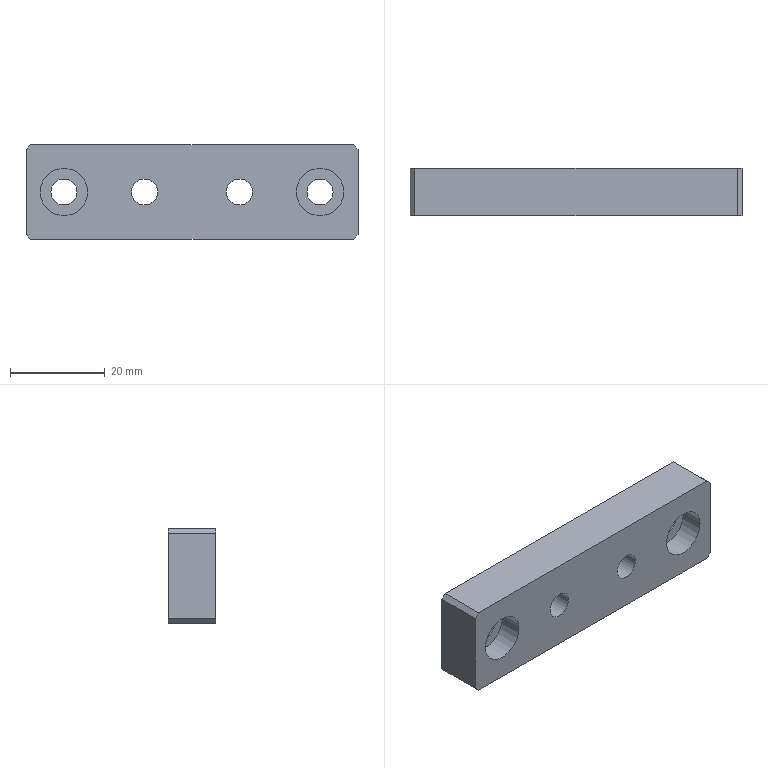Part | SolidWorks | features SplitBody 1 | 1 solid | 30 faces | box 70 x 10 x 20 mm | volume 11934 mm3 | cylinder 16 | plane 14 | commonest cylinder face diameters 5.5 x8 10 x8
STEP:
#1=CARTESIAN_POINT('',(508.292,46.908,-459.936));
#2=VERTEX_POINT('',#1);
#3=CARTESIAN_POINT('',(518.292,46.908,-459.936));
#4=VERTEX_POINT('',#3);
#5=CARTESIAN_POINT('',(513.292,46.908,-459.936));
#6=DIRECTION('',(0.,-1.,0.));
#7=DIRECTION('',(1.,0.,0.));
#8=AXIS2_PLACEMENT_3D('',#5,#6,#7);
#9=CIRCLE('',#8,5.);
#10=EDGE_CURVE('',#2,#4,#9,.T.);
#11=ORIENTED_EDGE('',*,*,#10,.F.);
#12=CARTESIAN_POINT('',(508.292,41.908,-459.936));
#13=VERTEX_POINT('',#12);
#14=CARTESIAN_POINT('',(508.292,41.908,-459.936));
#15=DIRECTION('',(0.,-1.,0.));
#16=VECTOR('',#15,1000.);
#17=LINE('',#14,#16);
#18=EDGE_CURVE('',#2,#13,#17,.T.);
#19=ORIENTED_EDGE('',*,*,#18,.T.);
#20=CARTESIAN_POINT('',(518.292,41.908,-459.936));
#21=VERTEX_POINT('',#20);
#22=CARTESIAN_POINT('',(513.292,41.908,-459.936));
#23=DIRECTION('',(0.,-1.,0.));
#24=DIRECTION('',(1.,0.,0.));
#25=AXIS2_PLACEMENT_3D('',#22,#23,#24);
#26=CIRCLE('',#25,5.);
#27=EDGE_CURVE('',#13,#21,#26,.T.);
#28=ORIENTED_EDGE('',*,*,#27,.T.);
#29=CARTESIAN_POINT('',(518.292,41.908,-459.936));
#30=DIRECTION('',(0.,-1.,0.));
#31=VECTOR('',#30,1000.);
#32=LINE('',#29,#31);
#33=EDGE_CURVE('',#4,#21,#32,.T.);
#34=ORIENTED_EDGE('',*,*,#33,.F.);
#35=EDGE_LOOP('',(#11,#19,#28,#34));
#36=FACE_OUTER_BOUND('',#35,.T.);
#37=CARTESIAN_POINT('',(513.292,41.908,-459.936));
#38=DIRECTION('',(0.,-1.,0.));
#39=DIRECTION('',(1.,0.,0.));
#40=AXIS2_PLACEMENT_3D('',#37,#38,#39);
#41=CYLINDRICAL_SURFACE('',#40,5.);
#42=ADVANCED_FACE('',(#36),#41,.F.);
#43=CARTESIAN_POINT('',(510.542,51.908,-459.936));
#44=VERTEX_POINT('',#43);
#45=CARTESIAN_POINT('',(516.042,51.908,-459.936));
#46=VERTEX_POINT('',#45);
#47=CARTESIAN_POINT('',(513.292,51.908,-459.936));
#48=DIRECTION('',(0.,-1.,0.));
#49=DIRECTION('',(1.,0.,0.));
#50=AXIS2_PLACEMENT_3D('',#47,#48,#49);
#51=CIRCLE('',#50,2.75);
#52=EDGE_CURVE('',#44,#46,#51,.T.);
#53=ORIENTED_EDGE('',*,*,#52,.F.);
#54=CARTESIAN_POINT('',(510.542,46.908,-459.936));
#55=VERTEX_POINT('',#54);
#56=CARTESIAN_POINT('',(510.542,41.908,-459.936));
#57=DIRECTION('',(0.,-1.,0.));
#58=VECTOR('',#57,1000.);
#59=LINE('',#56,#58);
#60=EDGE_CURVE('',#44,#55,#59,.T.);
#61=ORIENTED_EDGE('',*,*,#60,.T.);
#62=CARTESIAN_POINT('',(516.042,46.908,-459.936));
#63=VERTEX_POINT('',#62);
#64=CARTESIAN_POINT('',(513.292,46.908,-459.936));
#65=DIRECTION('',(0.,-1.,0.));
#66=DIRECTION('',(1.,0.,0.));
#67=AXIS2_PLACEMENT_3D('',#64,#65,#66);
#68=CIRCLE('',#67,2.75);
#69=EDGE_CURVE('',#55,#63,#68,.T.);
#70=ORIENTED_EDGE('',*,*,#69,.T.);
#71=CARTESIAN_POINT('',(516.042,41.908,-459.936));
#72=DIRECTION('',(0.,-1.,0.));
#73=VECTOR('',#72,1000.);
#74=LINE('',#71,#73);
#75=EDGE_CURVE('',#46,#63,#74,.T.);
#76=ORIENTED_EDGE('',*,*,#75,.F.);
#77=EDGE_LOOP('',(#53,#61,#70,#76));
#78=FACE_OUTER_BOUND('',#77,.T.);
#79=CARTESIAN_POINT('',(513.292,41.908,-459.936));
#80=DIRECTION('',(0.,-1.,0.));
#81=DIRECTION('',(1.,0.,0.));
#82=AXIS2_PLACEMENT_3D('',#79,#80,#81);
#83=CYLINDRICAL_SURFACE('',#82,2.75);
#84=ADVANCED_FACE('',(#78),#83,.F.);
#85=CARTESIAN_POINT('',(562.292,46.908,-459.936));
#86=VERTEX_POINT('',#85);
#87=CARTESIAN_POINT('',(572.292,46.908,-459.936));
#88=VERTEX_POINT('',#87);
#89=CARTESIAN_POINT('',(567.292,46.908,-459.936));
#90=DIRECTION('',(0.,-1.,0.));
#91=DIRECTION('',(1.,0.,0.));
#92=AXIS2_PLACEMENT_3D('',#89,#90,#91);
#93=CIRCLE('',#92,5.);
#94=EDGE_CURVE('',#86,#88,#93,.T.);
#95=ORIENTED_EDGE('',*,*,#94,.F.);
#96=CARTESIAN_POINT('',(562.292,41.908,-459.936));
#97=VERTEX_POINT('',#96);
#98=CARTESIAN_POINT('',(562.292,41.908,-459.936));
#99=DIRECTION('',(0.,-1.,0.));
#100=VECTOR('',#99,1000.);
#101=LINE('',#98,#100);
#102=EDGE_CURVE('',#86,#97,#101,.T.);
#103=ORIENTED_EDGE('',*,*,#102,.T.);
#104=CARTESIAN_POINT('',(572.292,41.908,-459.936));
#105=VERTEX_POINT('',#104);
#106=CARTESIAN_POINT('',(567.292,41.908,-459.936));
#107=DIRECTION('',(0.,-1.,0.));
#108=DIRECTION('',(1.,0.,0.));
#109=AXIS2_PLACEMENT_3D('',#106,#107,#108);
#110=CIRCLE('',#109,5.);
#111=EDGE_CURVE('',#97,#105,#110,.T.);
#112=ORIENTED_EDGE('',*,*,#111,.T.);
#113=CARTESIAN_POINT('',(572.292,41.908,-459.936));
#114=DIRECTION('',(0.,-1.,0.));
#115=VECTOR('',#114,1000.);
#116=LINE('',#113,#115);
#117=EDGE_CURVE('',#88,#105,#116,.T.);
#118=ORIENTED_EDGE('',*,*,#117,.F.);
#119=EDGE_LOOP('',(#95,#103,#112,#118));
#120=FACE_OUTER_BOUND('',#119,.T.);
#121=CARTESIAN_POINT('',(567.292,41.908,-459.936));
#122=DIRECTION('',(0.,-1.,0.));
#123=DIRECTION('',(1.,0.,0.));
#124=AXIS2_PLACEMENT_3D('',#121,#122,#123);
#125=CYLINDRICAL_SURFACE('',#124,5.);
#126=ADVANCED_FACE('',(#120),#125,.F.);
#127=CARTESIAN_POINT('',(564.542,51.908,-459.936));
#128=VERTEX_POINT('',#127);
#129=CARTESIAN_POINT('',(570.042,51.908,-459.936));
#130=VERTEX_POINT('',#129);
#131=CARTESIAN_POINT('',(567.292,51.908,-459.936));
#132=DIRECTION('',(0.,-1.,0.));
#133=DIRECTION('',(1.,0.,0.));
#134=AXIS2_PLACEMENT_3D('',#131,#132,#133);
#135=CIRCLE('',#134,2.75);
#136=EDGE_CURVE('',#128,#130,#135,.T.);
#137=ORIENTED_EDGE('',*,*,#136,.F.);
#138=CARTESIAN_POINT('',(564.542,46.908,-459.936));
#139=VERTEX_POINT('',#138);
#140=CARTESIAN_POINT('',(564.542,41.908,-459.936));
#141=DIRECTION('',(0.,-1.,0.));
#142=VECTOR('',#141,1000.);
#143=LINE('',#140,#142);
#144=EDGE_CURVE('',#128,#139,#143,.T.);
#145=ORIENTED_EDGE('',*,*,#144,.T.);
#146=CARTESIAN_POINT('',(570.042,46.908,-459.936));
#147=VERTEX_POINT('',#146);
#148=CARTESIAN_POINT('',(567.292,46.908,-459.936));
#149=DIRECTION('',(0.,-1.,0.));
#150=DIRECTION('',(1.,0.,0.));
#151=AXIS2_PLACEMENT_3D('',#148,#149,#150);
#152=CIRCLE('',#151,2.75);
#153=EDGE_CURVE('',#139,#147,#152,.T.);
#154=ORIENTED_EDGE('',*,*,#153,.T.);
#155=CARTESIAN_POINT('',(570.042,41.908,-459.936));
#156=DIRECTION('',(0.,-1.,0.));
#157=VECTOR('',#156,1000.);
#158=LINE('',#155,#157);
#159=EDGE_CURVE('',#130,#147,#158,.T.);
#160=ORIENTED_EDGE('',*,*,#159,.F.);
#161=EDGE_LOOP('',(#137,#145,#154,#160));
#162=FACE_OUTER_BOUND('',#161,.T.);
#163=CARTESIAN_POINT('',(567.292,41.908,-459.936));
#164=DIRECTION('',(0.,-1.,0.));
#165=DIRECTION('',(1.,0.,0.));
#166=AXIS2_PLACEMENT_3D('',#163,#164,#165);
#167=CYLINDRICAL_SURFACE('',#166,2.75);
#168=ADVANCED_FACE('',(#162),#167,.F.);
#169=CARTESIAN_POINT('',(555.292,46.908,-459.936));
#170=VERTEX_POINT('',#169);
#171=CARTESIAN_POINT('',(545.292,46.908,-459.936));
#172=VERTEX_POINT('',#171);
#173=CARTESIAN_POINT('',(550.292,46.908,-459.936));
#174=DIRECTION('',(0.,1.,0.));
#175=DIRECTION('',(-1.,0.,0.));
#176=AXIS2_PLACEMENT_3D('',#173,#174,#175);
#177=CIRCLE('',#176,5.);
#178=EDGE_CURVE('',#170,#172,#177,.T.);
#179=ORIENTED_EDGE('',*,*,#178,.F.);
#180=CARTESIAN_POINT('',(555.292,51.908,-459.936));
#181=VERTEX_POINT('',#180);
#182=CARTESIAN_POINT('',(555.292,51.908,-459.936));
#183=DIRECTION('',(0.,1.,0.));
#184=VECTOR('',#183,1000.);
#185=LINE('',#182,#184);
#186=EDGE_CURVE('',#170,#181,#185,.T.);
#187=ORIENTED_EDGE('',*,*,#186,.T.);
#188=CARTESIAN_POINT('',(545.292,51.908,-459.936));
#189=VERTEX_POINT('',#188);
#190=CARTESIAN_POINT('',(550.292,51.908,-459.936));
#191=DIRECTION('',(0.,1.,0.));
#192=DIRECTION('',(-1.,0.,0.));
#193=AXIS2_PLACEMENT_3D('',#190,#191,#192);
#194=CIRCLE('',#193,5.);
#195=EDGE_CURVE('',#181,#189,#194,.T.);
#196=ORIENTED_EDGE('',*,*,#195,.T.);
#197=CARTESIAN_POINT('',(545.292,51.908,-459.936));
#198=DIRECTION('',(0.,1.,0.));
#199=VECTOR('',#198,1000.);
#200=LINE('',#197,#199);
#201=EDGE_CURVE('',#172,#189,#200,.T.);
#202=ORIENTED_EDGE('',*,*,#201,.F.);
#203=EDGE_LOOP('',(#179,#187,#196,#202));
#204=FACE_OUTER_BOUND('',#203,.T.);
#205=CARTESIAN_POINT('',(550.292,51.908,-459.936));
#206=DIRECTION('',(0.,1.,0.));
#207=DIRECTION('',(-1.,0.,0.));
#208=AXIS2_PLACEMENT_3D('',#205,#206,#207);
#209=CYLINDRICAL_SURFACE('',#208,5.);
#210=ADVANCED_FACE('',(#204),#209,.F.);
#211=CARTESIAN_POINT('',(553.042,41.908,-459.936));
#212=VERTEX_POINT('',#211);
#213=CARTESIAN_POINT('',(547.542,41.908,-459.936));
#214=VERTEX_POINT('',#213);
#215=CARTESIAN_POINT('',(550.292,41.908,-459.936));
#216=DIRECTION('',(0.,1.,0.));
#217=DIRECTION('',(-1.,0.,0.));
#218=AXIS2_PLACEMENT_3D('',#215,#216,#217);
#219=CIRCLE('',#218,2.75);
#220=EDGE_CURVE('',#212,#214,#219,.T.);
#221=ORIENTED_EDGE('',*,*,#220,.F.);
#222=CARTESIAN_POINT('',(553.042,46.908,-459.936));
#223=VERTEX_POINT('',#222);
#224=CARTESIAN_POINT('',(553.042,51.908,-459.936));
#225=DIRECTION('',(0.,1.,0.));
#226=VECTOR('',#225,1000.);
#227=LINE('',#224,#226);
#228=EDGE_CURVE('',#212,#223,#227,.T.);
#229=ORIENTED_EDGE('',*,*,#228,.T.);
#230=CARTESIAN_POINT('',(547.542,46.908,-459.936));
#231=VERTEX_POINT('',#230);
#232=CARTESIAN_POINT('',(550.292,46.908,-459.936));
#233=DIRECTION('',(0.,1.,0.));
#234=DIRECTION('',(-1.,0.,0.));
#235=AXIS2_PLACEMENT_3D('',#232,#233,#234);
#236=CIRCLE('',#235,2.75);
#237=EDGE_CURVE('',#223,#231,#236,.T.);
#238=ORIENTED_EDGE('',*,*,#237,.T.);
#239=CARTESIAN_POINT('',(547.542,51.908,-459.936));
#240=DIRECTION('',(0.,1.,0.));
#241=VECTOR('',#240,1000.);
#242=LINE('',#239,#241);
#243=EDGE_CURVE('',#214,#231,#242,.T.);
#244=ORIENTED_EDGE('',*,*,#243,.F.);
#245=EDGE_LOOP('',(#221,#229,#238,#244));
#246=FACE_OUTER_BOUND('',#245,.T.);
#247=CARTESIAN_POINT('',(550.292,51.908,-459.936));
#248=DIRECTION('',(0.,1.,0.));
#249=DIRECTION('',(-1.,0.,0.));
#250=AXIS2_PLACEMENT_3D('',#247,#248,#249);
#251=CYLINDRICAL_SURFACE('',#250,2.75);
#252=ADVANCED_FACE('',(#246),#251,.F.);
#253=CARTESIAN_POINT('',(535.292,46.908,-459.936));
#254=VERTEX_POINT('',#253);
#255=CARTESIAN_POINT('',(525.292,46.908,-459.936));
#256=VERTEX_POINT('',#255);
#257=CARTESIAN_POINT('',(530.292,46.908,-459.936));
#258=DIRECTION('',(0.,1.,0.));
#259=DIRECTION('',(-1.,0.,0.));
#260=AXIS2_PLACEMENT_3D('',#257,#258,#259);
#261=CIRCLE('',#260,5.);
#262=EDGE_CURVE('',#254,#256,#261,.T.);
#263=ORIENTED_EDGE('',*,*,#262,.F.);
#264=CARTESIAN_POINT('',(535.292,51.908,-459.936));
#265=VERTEX_POINT('',#264);
#266=CARTESIAN_POINT('',(535.292,51.908,-459.936));
#267=DIRECTION('',(0.,1.,0.));
#268=VECTOR('',#267,1000.);
#269=LINE('',#266,#268);
#270=EDGE_CURVE('',#254,#265,#269,.T.);
#271=ORIENTED_EDGE('',*,*,#270,.T.);
#272=CARTESIAN_POINT('',(525.292,51.908,-459.936));
#273=VERTEX_POINT('',#272);
#274=CARTESIAN_POINT('',(530.292,51.908,-459.936));
#275=DIRECTION('',(0.,1.,0.));
#276=DIRECTION('',(-1.,0.,0.));
#277=AXIS2_PLACEMENT_3D('',#274,#275,#276);
#278=CIRCLE('',#277,5.);
#279=EDGE_CURVE('',#265,#273,#278,.T.);
#280=ORIENTED_EDGE('',*,*,#279,.T.);
#281=CARTESIAN_POINT('',(525.292,51.908,-459.936));
#282=DIRECTION('',(0.,1.,0.));
#283=VECTOR('',#282,1000.);
#284=LINE('',#281,#283);
#285=EDGE_CURVE('',#256,#273,#284,.T.);
#286=ORIENTED_EDGE('',*,*,#285,.F.);
#287=EDGE_LOOP('',(#263,#271,#280,#286));
#288=FACE_OUTER_BOUND('',#287,.T.);
#289=CARTESIAN_POINT('',(530.292,51.908,-459.936));
#290=DIRECTION('',(0.,1.,0.));
#291=DIRECTION('',(-1.,0.,0.));
#292=AXIS2_PLACEMENT_3D('',#289,#290,#291);
#293=CYLINDRICAL_SURFACE('',#292,5.);
#294=ADVANCED_FACE('',(#288),#293,.F.);
#295=CARTESIAN_POINT('',(533.042,41.908,-459.936));
#296=VERTEX_POINT('',#295);
#297=CARTESIAN_POINT('',(527.542,41.908,-459.936));
#298=VERTEX_POINT('',#297);
#299=CARTESIAN_POINT('',(530.292,41.908,-459.936));
#300=DIRECTION('',(0.,1.,0.));
#301=DIRECTION('',(-1.,0.,0.));
#302=AXIS2_PLACEMENT_3D('',#299,#300,#301);
#303=CIRCLE('',#302,2.75);
#304=EDGE_CURVE('',#296,#298,#303,.T.);
#305=ORIENTED_EDGE('',*,*,#304,.F.);
#306=CARTESIAN_POINT('',(533.042,46.908,-459.936));
#307=VERTEX_POINT('',#306);
#308=CARTESIAN_POINT('',(533.042,51.908,-459.936));
#309=DIRECTION('',(0.,1.,0.));
#310=VECTOR('',#309,1000.);
#311=LINE('',#308,#310);
#312=EDGE_CURVE('',#296,#307,#311,.T.);
#313=ORIENTED_EDGE('',*,*,#312,.T.);
#314=CARTESIAN_POINT('',(527.542,46.908,-459.936));
#315=VERTEX_POINT('',#314);
#316=CARTESIAN_POINT('',(530.292,46.908,-459.936));
#317=DIRECTION('',(0.,1.,0.));
#318=DIRECTION('',(-1.,0.,0.));
#319=AXIS2_PLACEMENT_3D('',#316,#317,#318);
#320=CIRCLE('',#319,2.75);
#321=EDGE_CURVE('',#307,#315,#320,.T.);
#322=ORIENTED_EDGE('',*,*,#321,.T.);
#323=CARTESIAN_POINT('',(527.542,51.908,-459.936));
#324=DIRECTION('',(0.,1.,0.));
#325=VECTOR('',#324,1000.);
#326=LINE('',#323,#325);
#327=EDGE_CURVE('',#298,#315,#326,.T.);
#328=ORIENTED_EDGE('',*,*,#327,.F.);
#329=EDGE_LOOP('',(#305,#313,#322,#328));
#330=FACE_OUTER_BOUND('',#329,.T.);
#331=CARTESIAN_POINT('',(530.292,51.908,-459.936));
#332=DIRECTION('',(0.,1.,0.));
#333=DIRECTION('',(-1.,0.,0.));
#334=AXIS2_PLACEMENT_3D('',#331,#332,#333);
#335=CYLINDRICAL_SURFACE('',#334,2.75);
#336=ADVANCED_FACE('',(#330),#335,.F.);
#337=CARTESIAN_POINT('',(505.292,51.908,-450.936));
#338=VERTEX_POINT('',#337);
#339=CARTESIAN_POINT('',(505.292,51.908,-468.936));
#340=VERTEX_POINT('',#339);
#341=CARTESIAN_POINT('',(505.292,51.908,-469.936));
#342=DIRECTION('',(0.,0.,-1.));
#343=VECTOR('',#342,1000.);
#344=LINE('',#341,#343);
#345=EDGE_CURVE('',#338,#340,#344,.T.);
#346=ORIENTED_EDGE('',*,*,#345,.T.);
#347=CARTESIAN_POINT('',(505.292,41.908,-468.936));
#348=VERTEX_POINT('',#347);
#349=CARTESIAN_POINT('',(505.292,41.908,-468.936));
#350=DIRECTION('',(0.,-1.,0.));
#351=VECTOR('',#350,1000.);
#352=LINE('',#349,#351);
#353=EDGE_CURVE('',#340,#348,#352,.T.);
#354=ORIENTED_EDGE('',*,*,#353,.T.);
#355=CARTESIAN_POINT('',(505.292,41.908,-450.936));
#356=VERTEX_POINT('',#355);
#357=CARTESIAN_POINT('',(505.292,41.908,-469.936));
#358=DIRECTION('',(0.,0.,-1.));
#359=VECTOR('',#358,1000.);
#360=LINE('',#357,#359);
#361=EDGE_CURVE('',#356,#348,#360,.T.);
#362=ORIENTED_EDGE('',*,*,#361,.F.);
#363=CARTESIAN_POINT('',(505.292,41.908,-450.936));
#364=DIRECTION('',(0.,1.,0.));
#365=VECTOR('',#364,1000.);
#366=LINE('',#363,#365);
#367=EDGE_CURVE('',#356,#338,#366,.T.);
#368=ORIENTED_EDGE('',*,*,#367,.T.);
#369=EDGE_LOOP('',(#346,#354,#362,#368));
#370=FACE_OUTER_BOUND('',#369,.T.);
#371=CARTESIAN_POINT('',(505.292,41.908,-469.936));
#372=DIRECTION('',(1.,0.,0.));
#373=DIRECTION('',(0.,1.,0.));
#374=AXIS2_PLACEMENT_3D('',#371,#372,#373);
#375=PLANE('',#374);
#376=ADVANCED_FACE('',(#370),#375,.F.);
#377=CARTESIAN_POINT('',(506.292,51.908,-469.936));
#378=VERTEX_POINT('',#377);
#379=CARTESIAN_POINT('',(574.292,51.908,-469.936));
#380=VERTEX_POINT('',#379);
#381=CARTESIAN_POINT('',(505.292,51.908,-469.936));
#382=DIRECTION('',(1.,0.,0.));
#383=VECTOR('',#382,1000.);
#384=LINE('',#381,#383);
#385=EDGE_CURVE('',#378,#380,#384,.T.);
#386=ORIENTED_EDGE('',*,*,#385,.T.);
#387=CARTESIAN_POINT('',(574.292,41.908,-469.936));
#388=VERTEX_POINT('',#387);
#389=CARTESIAN_POINT('',(574.292,41.908,-469.936));
#390=DIRECTION('',(0.,-1.,0.));
#391=VECTOR('',#390,1000.);
#392=LINE('',#389,#391);
#393=EDGE_CURVE('',#380,#388,#392,.T.);
#394=ORIENTED_EDGE('',*,*,#393,.T.);
#395=CARTESIAN_POINT('',(506.292,41.908,-469.936));
#396=VERTEX_POINT('',#395);
#397=CARTESIAN_POINT('',(505.292,41.908,-469.936));
#398=DIRECTION('',(1.,0.,0.));
#399=VECTOR('',#398,1000.);
#400=LINE('',#397,#399);
#401=EDGE_CURVE('',#396,#388,#400,.T.);
#402=ORIENTED_EDGE('',*,*,#401,.F.);
#403=CARTESIAN_POINT('',(506.292,41.908,-469.936));
#404=DIRECTION('',(0.,1.,0.));
#405=VECTOR('',#404,1000.);
#406=LINE('',#403,#405);
#407=EDGE_CURVE('',#396,#378,#406,.T.);
#408=ORIENTED_EDGE('',*,*,#407,.T.);
#409=EDGE_LOOP('',(#386,#394,#402,#408));
#410=FACE_OUTER_BOUND('',#409,.T.);
#411=CARTESIAN_POINT('',(505.292,41.908,-469.936));
#412=DIRECTION('',(0.,0.,1.));
#413=DIRECTION('',(0.,-1.,0.));
#414=AXIS2_PLACEMENT_3D('',#411,#412,#413);
#415=PLANE('',#414);
#416=ADVANCED_FACE('',(#410),#415,.F.);
#417=CARTESIAN_POINT('',(575.292,41.908,-468.936));
#418=VERTEX_POINT('',#417);
#419=CARTESIAN_POINT('',(575.292,41.908,-450.936));
#420=VERTEX_POINT('',#419);
#421=CARTESIAN_POINT('',(575.292,41.908,-469.936));
#422=DIRECTION('',(0.,0.,1.));
#423=VECTOR('',#422,1000.);
#424=LINE('',#421,#423);
#425=EDGE_CURVE('',#418,#420,#424,.T.);
#426=ORIENTED_EDGE('',*,*,#425,.F.);
#427=CARTESIAN_POINT('',(575.292,51.908,-468.936));
#428=VERTEX_POINT('',#427);
#429=CARTESIAN_POINT('',(575.292,41.908,-468.936));
#430=DIRECTION('',(0.,1.,0.));
#431=VECTOR('',#430,1000.);
#432=LINE('',#429,#431);
#433=EDGE_CURVE('',#418,#428,#432,.T.);
#434=ORIENTED_EDGE('',*,*,#433,.T.);
#435=CARTESIAN_POINT('',(575.292,51.908,-450.936));
#436=VERTEX_POINT('',#435);
#437=CARTESIAN_POINT('',(575.292,51.908,-469.936));
#438=DIRECTION('',(0.,0.,1.));
#439=VECTOR('',#438,1000.);
#440=LINE('',#437,#439);
#441=EDGE_CURVE('',#428,#436,#440,.T.);
#442=ORIENTED_EDGE('',*,*,#441,.T.);
#443=CARTESIAN_POINT('',(575.292,41.908,-450.936));
#444=DIRECTION('',(0.,-1.,0.));
#445=VECTOR('',#444,1000.);
#446=LINE('',#443,#445);
#447=EDGE_CURVE('',#436,#420,#446,.T.);
#448=ORIENTED_EDGE('',*,*,#447,.T.);
#449=EDGE_LOOP('',(#426,#434,#442,#448));
#450=FACE_OUTER_BOUND('',#449,.T.);
#451=CARTESIAN_POINT('',(575.292,41.908,-469.936));
#452=DIRECTION('',(-1.,0.,0.));
#453=DIRECTION('',(0.,-1.,0.));
#454=AXIS2_PLACEMENT_3D('',#451,#452,#453);
#455=PLANE('',#454);
#456=ADVANCED_FACE('',(#450),#455,.F.);
#457=CARTESIAN_POINT('',(574.292,41.908,-449.936));
#458=VERTEX_POINT('',#457);
#459=CARTESIAN_POINT('',(506.292,41.908,-449.936));
#460=VERTEX_POINT('',#459);
#461=CARTESIAN_POINT('',(505.292,41.908,-449.936));
#462=DIRECTION('',(-1.,0.,0.));
#463=VECTOR('',#462,1000.);
#464=LINE('',#461,#463);
#465=EDGE_CURVE('',#458,#460,#464,.T.);
#466=ORIENTED_EDGE('',*,*,#465,.F.);
#467=CARTESIAN_POINT('',(574.292,51.908,-449.936));
#468=VERTEX_POINT('',#467);
#469=CARTESIAN_POINT('',(574.292,41.908,-449.936));
#470=DIRECTION('',(0.,1.,0.));
#471=VECTOR('',#470,1000.);
#472=LINE('',#469,#471);
#473=EDGE_CURVE('',#458,#468,#472,.T.);
#474=ORIENTED_EDGE('',*,*,#473,.T.);
#475=CARTESIAN_POINT('',(506.292,51.908,-449.936));
#476=VERTEX_POINT('',#475);
#477=CARTESIAN_POINT('',(505.292,51.908,-449.936));
#478=DIRECTION('',(-1.,0.,0.));
#479=VECTOR('',#478,1000.);
#480=LINE('',#477,#479);
#481=EDGE_CURVE('',#468,#476,#480,.T.);
#482=ORIENTED_EDGE('',*,*,#481,.T.);
#483=CARTESIAN_POINT('',(506.292,41.908,-449.936));
#484=DIRECTION('',(0.,-1.,0.));
#485=VECTOR('',#484,1000.);
#486=LINE('',#483,#485);
#487=EDGE_CURVE('',#476,#460,#486,.T.);
#488=ORIENTED_EDGE('',*,*,#487,.T.);
#489=EDGE_LOOP('',(#466,#474,#482,#488));
#490=FACE_OUTER_BOUND('',#489,.T.);
#491=CARTESIAN_POINT('',(505.292,41.908,-449.936));
#492=DIRECTION('',(0.,0.,-1.));
#493=DIRECTION('',(0.,1.,0.));
#494=AXIS2_PLACEMENT_3D('',#491,#492,#493);
#495=PLANE('',#494);
#496=ADVANCED_FACE('',(#490),#495,.F.);
#497=CARTESIAN_POINT('',(513.292,41.908,-459.936));
#498=DIRECTION('',(0.,-1.,0.));
#499=DIRECTION('',(1.,0.,0.));
#500=AXIS2_PLACEMENT_3D('',#497,#498,#499);
#501=CIRCLE('',#500,5.);
#502=EDGE_CURVE('',#21,#13,#501,.T.);
#503=ORIENTED_EDGE('',*,*,#502,.F.);
#504=ORIENTED_EDGE('',*,*,#27,.F.);
#505=EDGE_LOOP('',(#503,#504));
#506=FACE_BOUND('',#505,.T.);
#507=CARTESIAN_POINT('',(567.292,41.908,-459.936));
#508=DIRECTION('',(0.,-1.,0.));
#509=DIRECTION('',(1.,0.,0.));
#510=AXIS2_PLACEMENT_3D('',#507,#508,#509);
#511=CIRCLE('',#510,5.);
#512=EDGE_CURVE('',#105,#97,#511,.T.);
#513=ORIENTED_EDGE('',*,*,#512,.F.);
#514=ORIENTED_EDGE('',*,*,#111,.F.);
#515=EDGE_LOOP('',(#513,#514));
#516=FACE_BOUND('',#515,.T.);
#517=CARTESIAN_POINT('',(550.292,41.908,-459.936));
#518=DIRECTION('',(0.,1.,0.));
#519=DIRECTION('',(-1.,0.,0.));
#520=AXIS2_PLACEMENT_3D('',#517,#518,#519);
#521=CIRCLE('',#520,2.75);
#522=EDGE_CURVE('',#214,#212,#521,.T.);
#523=ORIENTED_EDGE('',*,*,#522,.T.);
#524=ORIENTED_EDGE('',*,*,#220,.T.);
#525=EDGE_LOOP('',(#523,#524));
#526=FACE_BOUND('',#525,.T.);
#527=CARTESIAN_POINT('',(530.292,41.908,-459.936));
#528=DIRECTION('',(0.,1.,0.));
#529=DIRECTION('',(-1.,0.,0.));
#530=AXIS2_PLACEMENT_3D('',#527,#528,#529);
#531=CIRCLE('',#530,2.75);
#532=EDGE_CURVE('',#298,#296,#531,.T.);
#533=ORIENTED_EDGE('',*,*,#532,.T.);
#534=ORIENTED_EDGE('',*,*,#304,.T.);
#535=EDGE_LOOP('',(#533,#534));
#536=FACE_BOUND('',#535,.T.);
#537=ORIENTED_EDGE('',*,*,#401,.T.);
#538=CARTESIAN_POINT('',(575.292,41.908,-468.936));
#539=DIRECTION('',(0.7071,0.,0.7071));
#540=VECTOR('',#539,1000.);
#541=LINE('',#538,#540);
#542=EDGE_CURVE('',#388,#418,#541,.T.);
#543=ORIENTED_EDGE('',*,*,#542,.T.);
#544=ORIENTED_EDGE('',*,*,#425,.T.);
#545=CARTESIAN_POINT('',(574.292,41.908,-449.936));
#546=DIRECTION('',(-0.7071,0.,0.7071));
#547=VECTOR('',#546,1000.);
#548=LINE('',#545,#547);
#549=EDGE_CURVE('',#420,#458,#548,.T.);
#550=ORIENTED_EDGE('',*,*,#549,.T.);
#551=ORIENTED_EDGE('',*,*,#465,.T.);
#552=CARTESIAN_POINT('',(505.292,41.908,-450.936));
#553=DIRECTION('',(-0.7071,0.,-0.7071));
#554=VECTOR('',#553,1000.);
#555=LINE('',#552,#554);
#556=EDGE_CURVE('',#460,#356,#555,.T.);
#557=ORIENTED_EDGE('',*,*,#556,.T.);
#558=ORIENTED_EDGE('',*,*,#361,.T.);
#559=CARTESIAN_POINT('',(506.292,41.908,-469.936));
#560=DIRECTION('',(0.7071,0.,-0.7071));
#561=VECTOR('',#560,1000.);
#562=LINE('',#559,#561);
#563=EDGE_CURVE('',#348,#396,#562,.T.);
#564=ORIENTED_EDGE('',*,*,#563,.T.);
#565=EDGE_LOOP('',(#537,#543,#544,#550,#551,#557,#558,#564));
#566=FACE_OUTER_BOUND('',#565,.T.);
#567=CARTESIAN_POINT('',(505.292,41.908,-449.936));
#568=DIRECTION('',(0.,1.,0.));
#569=DIRECTION('',(-1.,0.,0.));
#570=AXIS2_PLACEMENT_3D('',#567,#568,#569);
#571=PLANE('',#570);
#572=ADVANCED_FACE('',(#506,#516,#526,#536,#566),#571,.F.);
#573=CARTESIAN_POINT('',(513.292,51.908,-459.936));
#574=DIRECTION('',(0.,-1.,0.));
#575=DIRECTION('',(1.,0.,0.));
#576=AXIS2_PLACEMENT_3D('',#573,#574,#575);
#577=CIRCLE('',#576,2.75);
#578=EDGE_CURVE('',#46,#44,#577,.T.);
#579=ORIENTED_EDGE('',*,*,#578,.T.);
#580=ORIENTED_EDGE('',*,*,#52,.T.);
#581=EDGE_LOOP('',(#579,#580));
#582=FACE_BOUND('',#581,.T.);
#583=CARTESIAN_POINT('',(567.292,51.908,-459.936));
#584=DIRECTION('',(0.,-1.,0.));
#585=DIRECTION('',(1.,0.,0.));
#586=AXIS2_PLACEMENT_3D('',#583,#584,#585);
#587=CIRCLE('',#586,2.75);
#588=EDGE_CURVE('',#130,#128,#587,.T.);
#589=ORIENTED_EDGE('',*,*,#588,.T.);
#590=ORIENTED_EDGE('',*,*,#136,.T.);
#591=EDGE_LOOP('',(#589,#590));
#592=FACE_BOUND('',#591,.T.);
#593=CARTESIAN_POINT('',(550.292,51.908,-459.936));
#594=DIRECTION('',(0.,1.,0.));
#595=DIRECTION('',(-1.,0.,0.));
#596=AXIS2_PLACEMENT_3D('',#593,#594,#595);
#597=CIRCLE('',#596,5.);
#598=EDGE_CURVE('',#189,#181,#597,.T.);
#599=ORIENTED_EDGE('',*,*,#598,.F.);
#600=ORIENTED_EDGE('',*,*,#195,.F.);
#601=EDGE_LOOP('',(#599,#600));
#602=FACE_BOUND('',#601,.T.);
#603=CARTESIAN_POINT('',(530.292,51.908,-459.936));
#604=DIRECTION('',(0.,1.,0.));
#605=DIRECTION('',(-1.,0.,0.));
#606=AXIS2_PLACEMENT_3D('',#603,#604,#605);
#607=CIRCLE('',#606,5.);
#608=EDGE_CURVE('',#273,#265,#607,.T.);
#609=ORIENTED_EDGE('',*,*,#608,.F.);
#610=ORIENTED_EDGE('',*,*,#279,.F.);
#611=EDGE_LOOP('',(#609,#610));
#612=FACE_BOUND('',#611,.T.);
#613=ORIENTED_EDGE('',*,*,#441,.F.);
#614=CARTESIAN_POINT('',(549.792,51.908,-494.436));
#615=DIRECTION('',(-0.7071,0.,-0.7071));
#616=VECTOR('',#615,1000.);
#617=LINE('',#614,#616);
#618=EDGE_CURVE('',#428,#380,#617,.T.);
#619=ORIENTED_EDGE('',*,*,#618,.T.);
#620=ORIENTED_EDGE('',*,*,#385,.F.);
#621=CARTESIAN_POINT('',(495.792,51.908,-459.436));
#622=DIRECTION('',(-0.7071,0.,0.7071));
#623=VECTOR('',#622,1000.);
#624=LINE('',#621,#623);
#625=EDGE_CURVE('',#378,#340,#624,.T.);
#626=ORIENTED_EDGE('',*,*,#625,.T.);
#627=ORIENTED_EDGE('',*,*,#345,.F.);
#628=CARTESIAN_POINT('',(505.792,51.908,-450.436));
#629=DIRECTION('',(0.7071,0.,0.7071));
#630=VECTOR('',#629,1000.);
#631=LINE('',#628,#630);
#632=EDGE_CURVE('',#338,#476,#631,.T.);
#633=ORIENTED_EDGE('',*,*,#632,.T.);
#634=ORIENTED_EDGE('',*,*,#481,.F.);
#635=CARTESIAN_POINT('',(539.792,51.908,-415.436));
#636=DIRECTION('',(0.7071,0.,-0.7071));
#637=VECTOR('',#636,1000.);
#638=LINE('',#635,#637);
#639=EDGE_CURVE('',#468,#436,#638,.T.);
#640=ORIENTED_EDGE('',*,*,#639,.T.);
#641=EDGE_LOOP('',(#613,#619,#620,#626,#627,#633,#634,#640));
#642=FACE_OUTER_BOUND('',#641,.T.);
#643=CARTESIAN_POINT('',(505.292,51.908,-449.936));
#644=DIRECTION('',(0.,1.,0.));
#645=DIRECTION('',(-1.,0.,0.));
#646=AXIS2_PLACEMENT_3D('',#643,#644,#645);
#647=PLANE('',#646);
#648=ADVANCED_FACE('',(#582,#592,#602,#612,#642),#647,.T.);
#649=ORIENTED_EDGE('',*,*,#312,.F.);
#650=ORIENTED_EDGE('',*,*,#532,.F.);
#651=ORIENTED_EDGE('',*,*,#327,.T.);
#652=CARTESIAN_POINT('',(530.292,46.908,-459.936));
#653=DIRECTION('',(0.,1.,0.));
#654=DIRECTION('',(-1.,0.,0.));
#655=AXIS2_PLACEMENT_3D('',#652,#653,#654);
#656=CIRCLE('',#655,2.75);
#657=EDGE_CURVE('',#315,#307,#656,.T.);
#658=ORIENTED_EDGE('',*,*,#657,.T.);
#659=EDGE_LOOP('',(#649,#650,#651,#658));
#660=FACE_OUTER_BOUND('',#659,.T.);
#661=CARTESIAN_POINT('',(530.292,51.908,-459.936));
#662=DIRECTION('',(0.,1.,0.));
#663=DIRECTION('',(-1.,0.,0.));
#664=AXIS2_PLACEMENT_3D('',#661,#662,#663);
#665=CYLINDRICAL_SURFACE('',#664,2.75);
#666=ADVANCED_FACE('',(#660),#665,.F.);
#667=ORIENTED_EDGE('',*,*,#657,.F.);
#668=ORIENTED_EDGE('',*,*,#321,.F.);
#669=EDGE_LOOP('',(#667,#668));
#670=FACE_BOUND('',#669,.T.);
#671=CARTESIAN_POINT('',(530.292,46.908,-459.936));
#672=DIRECTION('',(0.,1.,0.));
#673=DIRECTION('',(-1.,0.,0.));
#674=AXIS2_PLACEMENT_3D('',#671,#672,#673);
#675=CIRCLE('',#674,5.);
#676=EDGE_CURVE('',#256,#254,#675,.T.);
#677=ORIENTED_EDGE('',*,*,#676,.T.);
#678=ORIENTED_EDGE('',*,*,#262,.T.);
#679=EDGE_LOOP('',(#677,#678));
#680=FACE_OUTER_BOUND('',#679,.T.);
#681=CARTESIAN_POINT('',(533.042,46.908,-459.936));
#682=DIRECTION('',(0.,-1.,0.));
#683=DIRECTION('',(1.,0.,0.));
#684=AXIS2_PLACEMENT_3D('',#681,#682,#683);
#685=PLANE('',#684);
#686=ADVANCED_FACE('',(#670,#680),#685,.F.);
#687=ORIENTED_EDGE('',*,*,#270,.F.);
#688=ORIENTED_EDGE('',*,*,#676,.F.);
#689=ORIENTED_EDGE('',*,*,#285,.T.);
#690=ORIENTED_EDGE('',*,*,#608,.T.);
#691=EDGE_LOOP('',(#687,#688,#689,#690));
#692=FACE_OUTER_BOUND('',#691,.T.);
#693=CARTESIAN_POINT('',(530.292,51.908,-459.936));
#694=DIRECTION('',(0.,1.,0.));
#695=DIRECTION('',(-1.,0.,0.));
#696=AXIS2_PLACEMENT_3D('',#693,#694,#695);
#697=CYLINDRICAL_SURFACE('',#696,5.);
#698=ADVANCED_FACE('',(#692),#697,.F.);
#699=ORIENTED_EDGE('',*,*,#228,.F.);
#700=ORIENTED_EDGE('',*,*,#522,.F.);
#701=ORIENTED_EDGE('',*,*,#243,.T.);
#702=CARTESIAN_POINT('',(550.292,46.908,-459.936));
#703=DIRECTION('',(0.,1.,0.));
#704=DIRECTION('',(-1.,0.,0.));
#705=AXIS2_PLACEMENT_3D('',#702,#703,#704);
#706=CIRCLE('',#705,2.75);
#707=EDGE_CURVE('',#231,#223,#706,.T.);
#708=ORIENTED_EDGE('',*,*,#707,.T.);
#709=EDGE_LOOP('',(#699,#700,#701,#708));
#710=FACE_OUTER_BOUND('',#709,.T.);
#711=CARTESIAN_POINT('',(550.292,51.908,-459.936));
#712=DIRECTION('',(0.,1.,0.));
#713=DIRECTION('',(-1.,0.,0.));
#714=AXIS2_PLACEMENT_3D('',#711,#712,#713);
#715=CYLINDRICAL_SURFACE('',#714,2.75);
#716=ADVANCED_FACE('',(#710),#715,.F.);
#717=ORIENTED_EDGE('',*,*,#707,.F.);
#718=ORIENTED_EDGE('',*,*,#237,.F.);
#719=EDGE_LOOP('',(#717,#718));
#720=FACE_BOUND('',#719,.T.);
#721=CARTESIAN_POINT('',(550.292,46.908,-459.936));
#722=DIRECTION('',(0.,1.,0.));
#723=DIRECTION('',(-1.,0.,0.));
#724=AXIS2_PLACEMENT_3D('',#721,#722,#723);
#725=CIRCLE('',#724,5.);
#726=EDGE_CURVE('',#172,#170,#725,.T.);
#727=ORIENTED_EDGE('',*,*,#726,.T.);
#728=ORIENTED_EDGE('',*,*,#178,.T.);
#729=EDGE_LOOP('',(#727,#728));
#730=FACE_OUTER_BOUND('',#729,.T.);
#731=CARTESIAN_POINT('',(553.042,46.908,-459.936));
#732=DIRECTION('',(0.,-1.,0.));
#733=DIRECTION('',(1.,0.,0.));
#734=AXIS2_PLACEMENT_3D('',#731,#732,#733);
#735=PLANE('',#734);
#736=ADVANCED_FACE('',(#720,#730),#735,.F.);
#737=ORIENTED_EDGE('',*,*,#186,.F.);
#738=ORIENTED_EDGE('',*,*,#726,.F.);
#739=ORIENTED_EDGE('',*,*,#201,.T.);
#740=ORIENTED_EDGE('',*,*,#598,.T.);
#741=EDGE_LOOP('',(#737,#738,#739,#740));
#742=FACE_OUTER_BOUND('',#741,.T.);
#743=CARTESIAN_POINT('',(550.292,51.908,-459.936));
#744=DIRECTION('',(0.,1.,0.));
#745=DIRECTION('',(-1.,0.,0.));
#746=AXIS2_PLACEMENT_3D('',#743,#744,#745);
#747=CYLINDRICAL_SURFACE('',#746,5.);
#748=ADVANCED_FACE('',(#742),#747,.F.);
#749=ORIENTED_EDGE('',*,*,#144,.F.);
#750=ORIENTED_EDGE('',*,*,#588,.F.);
#751=ORIENTED_EDGE('',*,*,#159,.T.);
#752=CARTESIAN_POINT('',(567.292,46.908,-459.936));
#753=DIRECTION('',(0.,-1.,0.));
#754=DIRECTION('',(1.,0.,0.));
#755=AXIS2_PLACEMENT_3D('',#752,#753,#754);
#756=CIRCLE('',#755,2.75);
#757=EDGE_CURVE('',#147,#139,#756,.T.);
#758=ORIENTED_EDGE('',*,*,#757,.T.);
#759=EDGE_LOOP('',(#749,#750,#751,#758));
#760=FACE_OUTER_BOUND('',#759,.T.);
#761=CARTESIAN_POINT('',(567.292,41.908,-459.936));
#762=DIRECTION('',(0.,-1.,0.));
#763=DIRECTION('',(1.,0.,0.));
#764=AXIS2_PLACEMENT_3D('',#761,#762,#763);
#765=CYLINDRICAL_SURFACE('',#764,2.75);
#766=ADVANCED_FACE('',(#760),#765,.F.);
#767=ORIENTED_EDGE('',*,*,#757,.F.);
#768=ORIENTED_EDGE('',*,*,#153,.F.);
#769=EDGE_LOOP('',(#767,#768));
#770=FACE_BOUND('',#769,.T.);
#771=CARTESIAN_POINT('',(567.292,46.908,-459.936));
#772=DIRECTION('',(0.,-1.,0.));
#773=DIRECTION('',(1.,0.,0.));
#774=AXIS2_PLACEMENT_3D('',#771,#772,#773);
#775=CIRCLE('',#774,5.);
#776=EDGE_CURVE('',#88,#86,#775,.T.);
#777=ORIENTED_EDGE('',*,*,#776,.T.);
#778=ORIENTED_EDGE('',*,*,#94,.T.);
#779=EDGE_LOOP('',(#777,#778));
#780=FACE_OUTER_BOUND('',#779,.T.);
#781=CARTESIAN_POINT('',(570.042,46.908,-459.936));
#782=DIRECTION('',(0.,1.,0.));
#783=DIRECTION('',(-1.,0.,0.));
#784=AXIS2_PLACEMENT_3D('',#781,#782,#783);
#785=PLANE('',#784);
#786=ADVANCED_FACE('',(#770,#780),#785,.F.);
#787=ORIENTED_EDGE('',*,*,#102,.F.);
#788=ORIENTED_EDGE('',*,*,#776,.F.);
#789=ORIENTED_EDGE('',*,*,#117,.T.);
#790=ORIENTED_EDGE('',*,*,#512,.T.);
#791=EDGE_LOOP('',(#787,#788,#789,#790));
#792=FACE_OUTER_BOUND('',#791,.T.);
#793=CARTESIAN_POINT('',(567.292,41.908,-459.936));
#794=DIRECTION('',(0.,-1.,0.));
#795=DIRECTION('',(1.,0.,0.));
#796=AXIS2_PLACEMENT_3D('',#793,#794,#795);
#797=CYLINDRICAL_SURFACE('',#796,5.);
#798=ADVANCED_FACE('',(#792),#797,.F.);
#799=ORIENTED_EDGE('',*,*,#60,.F.);
#800=ORIENTED_EDGE('',*,*,#578,.F.);
#801=ORIENTED_EDGE('',*,*,#75,.T.);
#802=CARTESIAN_POINT('',(513.292,46.908,-459.936));
#803=DIRECTION('',(0.,-1.,0.));
#804=DIRECTION('',(1.,0.,0.));
#805=AXIS2_PLACEMENT_3D('',#802,#803,#804);
#806=CIRCLE('',#805,2.75);
#807=EDGE_CURVE('',#63,#55,#806,.T.);
#808=ORIENTED_EDGE('',*,*,#807,.T.);
#809=EDGE_LOOP('',(#799,#800,#801,#808));
#810=FACE_OUTER_BOUND('',#809,.T.);
#811=CARTESIAN_POINT('',(513.292,41.908,-459.936));
#812=DIRECTION('',(0.,-1.,0.));
#813=DIRECTION('',(1.,0.,0.));
#814=AXIS2_PLACEMENT_3D('',#811,#812,#813);
#815=CYLINDRICAL_SURFACE('',#814,2.75);
#816=ADVANCED_FACE('',(#810),#815,.F.);
#817=ORIENTED_EDGE('',*,*,#807,.F.);
#818=ORIENTED_EDGE('',*,*,#69,.F.);
#819=EDGE_LOOP('',(#817,#818));
#820=FACE_BOUND('',#819,.T.);
#821=CARTESIAN_POINT('',(513.292,46.908,-459.936));
#822=DIRECTION('',(0.,-1.,0.));
#823=DIRECTION('',(1.,0.,0.));
#824=AXIS2_PLACEMENT_3D('',#821,#822,#823);
#825=CIRCLE('',#824,5.);
#826=EDGE_CURVE('',#4,#2,#825,.T.);
#827=ORIENTED_EDGE('',*,*,#826,.T.);
#828=ORIENTED_EDGE('',*,*,#10,.T.);
#829=EDGE_LOOP('',(#827,#828));
#830=FACE_OUTER_BOUND('',#829,.T.);
#831=CARTESIAN_POINT('',(516.042,46.908,-459.936));
#832=DIRECTION('',(0.,1.,0.));
#833=DIRECTION('',(-1.,0.,0.));
#834=AXIS2_PLACEMENT_3D('',#831,#832,#833);
#835=PLANE('',#834);
#836=ADVANCED_FACE('',(#820,#830),#835,.F.);
#837=ORIENTED_EDGE('',*,*,#18,.F.);
#838=ORIENTED_EDGE('',*,*,#826,.F.);
#839=ORIENTED_EDGE('',*,*,#33,.T.);
#840=ORIENTED_EDGE('',*,*,#502,.T.);
#841=EDGE_LOOP('',(#837,#838,#839,#840));
#842=FACE_OUTER_BOUND('',#841,.T.);
#843=CARTESIAN_POINT('',(513.292,41.908,-459.936));
#844=DIRECTION('',(0.,-1.,0.));
#845=DIRECTION('',(1.,0.,0.));
#846=AXIS2_PLACEMENT_3D('',#843,#844,#845);
#847=CYLINDRICAL_SURFACE('',#846,5.);
#848=ADVANCED_FACE('',(#842),#847,.F.);
#849=ORIENTED_EDGE('',*,*,#542,.F.);
#850=ORIENTED_EDGE('',*,*,#393,.F.);
#851=ORIENTED_EDGE('',*,*,#618,.F.);
#852=ORIENTED_EDGE('',*,*,#433,.F.);
#853=EDGE_LOOP('',(#849,#850,#851,#852));
#854=FACE_OUTER_BOUND('',#853,.T.);
#855=CARTESIAN_POINT('',(575.292,41.908,-468.936));
#856=DIRECTION('',(-0.7071,0.,0.7071));
#857=DIRECTION('',(-0.7071,0.,-0.7071));
#858=AXIS2_PLACEMENT_3D('',#855,#856,#857);
#859=PLANE('',#858);
#860=ADVANCED_FACE('',(#854),#859,.F.);
#861=ORIENTED_EDGE('',*,*,#563,.F.);
#862=ORIENTED_EDGE('',*,*,#353,.F.);
#863=ORIENTED_EDGE('',*,*,#625,.F.);
#864=ORIENTED_EDGE('',*,*,#407,.F.);
#865=EDGE_LOOP('',(#861,#862,#863,#864));
#866=FACE_OUTER_BOUND('',#865,.T.);
#867=CARTESIAN_POINT('',(506.292,41.908,-469.936));
#868=DIRECTION('',(0.7071,0.,0.7071));
#869=DIRECTION('',(-0.7071,0.,0.7071));
#870=AXIS2_PLACEMENT_3D('',#867,#868,#869);
#871=PLANE('',#870);
#872=ADVANCED_FACE('',(#866),#871,.F.);
#873=ORIENTED_EDGE('',*,*,#549,.F.);
#874=ORIENTED_EDGE('',*,*,#447,.F.);
#875=ORIENTED_EDGE('',*,*,#639,.F.);
#876=ORIENTED_EDGE('',*,*,#473,.F.);
#877=EDGE_LOOP('',(#873,#874,#875,#876));
#878=FACE_OUTER_BOUND('',#877,.T.);
#879=CARTESIAN_POINT('',(574.292,41.908,-449.936));
#880=DIRECTION('',(-0.7071,0.,-0.7071));
#881=DIRECTION('',(0.7071,0.,-0.7071));
#882=AXIS2_PLACEMENT_3D('',#879,#880,#881);
#883=PLANE('',#882);
#884=ADVANCED_FACE('',(#878),#883,.F.);
#885=ORIENTED_EDGE('',*,*,#556,.F.);
#886=ORIENTED_EDGE('',*,*,#487,.F.);
#887=ORIENTED_EDGE('',*,*,#632,.F.);
#888=ORIENTED_EDGE('',*,*,#367,.F.);
#889=EDGE_LOOP('',(#885,#886,#887,#888));
#890=FACE_OUTER_BOUND('',#889,.T.);
#891=CARTESIAN_POINT('',(505.292,41.908,-450.936));
#892=DIRECTION('',(0.7071,0.,-0.7071));
#893=DIRECTION('',(0.7071,0.,0.7071));
#894=AXIS2_PLACEMENT_3D('',#891,#892,#893);
#895=PLANE('',#894);
#896=ADVANCED_FACE('',(#890),#895,.F.);
#897=CLOSED_SHELL('',(#42,#84,#126,#168,#210,#252,#294,#336,#376,#416,#456,#496,#572,#648,#666,#686,#698,#716,#736,#748,#766,#786,#798,#816,#836,#848,#860,#872,#884,#896));
#898=MANIFOLD_SOLID_BREP('',#897);
#899=CARTESIAN_POINT('',(0.,0.,0.));
#900=DIRECTION('',(0.,0.,1.));
#901=DIRECTION('',(1.,0.,0.));
#902=AXIS2_PLACEMENT_3D('',#899,#900,#901);
#903=(LENGTH_UNIT()NAMED_UNIT(*)SI_UNIT(.MILLI.,.METRE.));
#904=UNCERTAINTY_MEASURE_WITH_UNIT(LENGTH_MEASURE(0.00001),#903,'','');
#905=(NAMED_UNIT(*)PLANE_ANGLE_UNIT()SI_UNIT($,.RADIAN.));
#906=(NAMED_UNIT(*)SI_UNIT($,.STERADIAN.)SOLID_ANGLE_UNIT());
#907=(GEOMETRIC_REPRESENTATION_CONTEXT(3)GLOBAL_UNCERTAINTY_ASSIGNED_CONTEXT((#904))GLOBAL_UNIT_ASSIGNED_CONTEXT((#903,#905,#906))REPRESENTATION_CONTEXT('',''));
#908=ADVANCED_BREP_SHAPE_REPRESENTATION('',(#898,#902),#907);